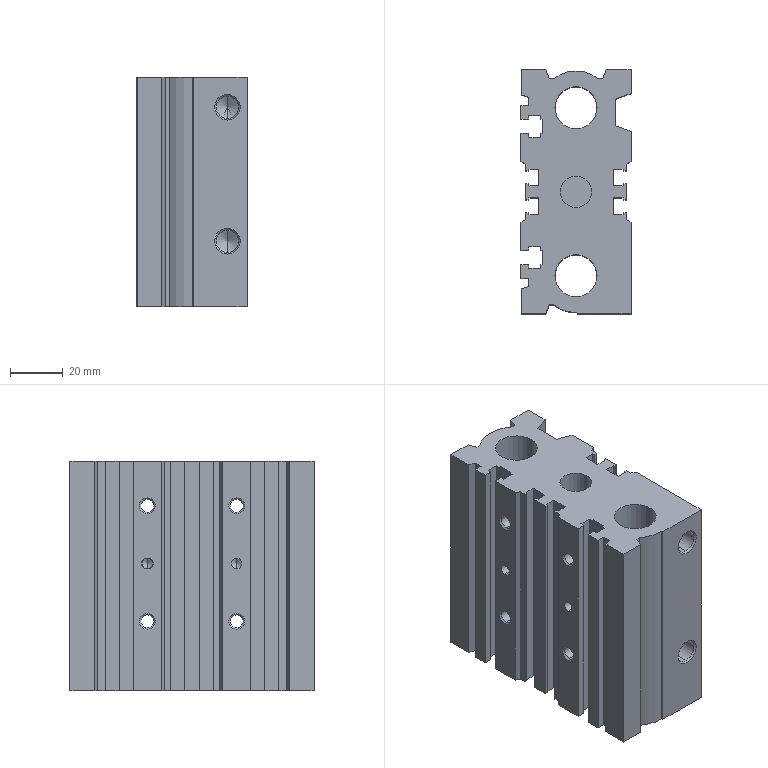Part | SolidWorks | features BaseBody 1 | 1 solid | 215 faces | box 42 x 93 x 87.5 mm | volume 227496 mm3 | plane 113 | cylinder 62 | cone 40 | commonest cylinder face diameters 4.917 x16 4 x12 5.4 x8 8.566 x8 9.5 x8 16 x4